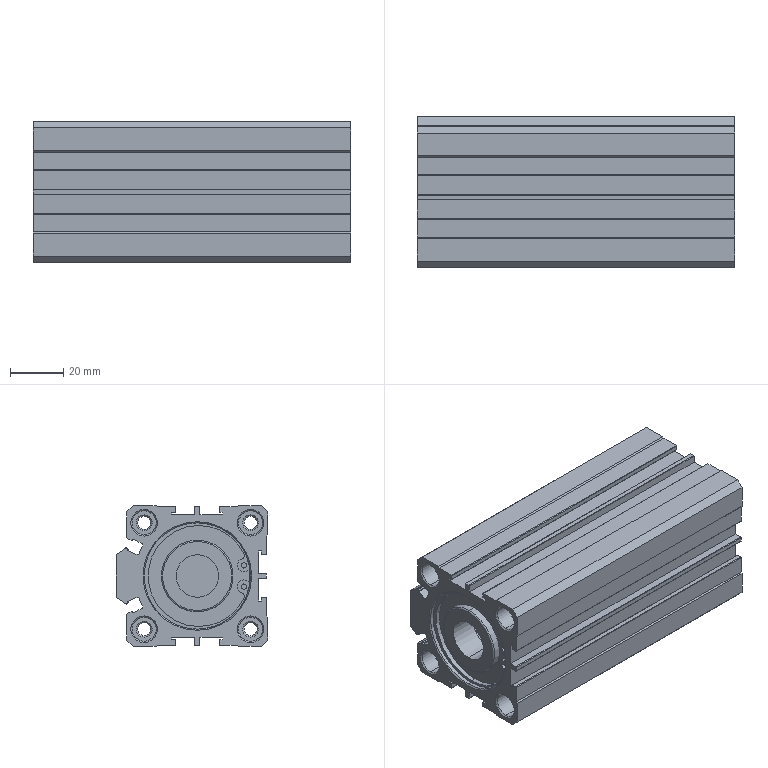Part | STEP file | ACQS_40x8080_b | 1 solid | 246 faces | box 119.5 x 57 x 53 mm | volume 166175 mm3 | cylinder 108 | plane 92 | cone 44 | torus 2 | commonest cylinder face diameters 0.4 x35 9 x16 0.8 x15 2 x8 4.917 x8 40 x6